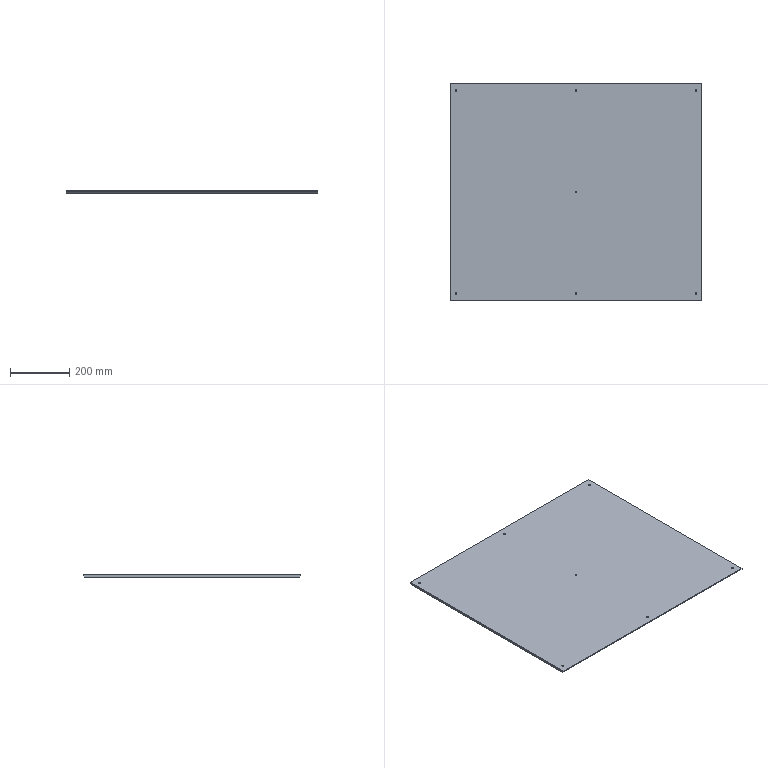Part | SolidWorks | features ICE 4, Chamfer 1, Extrusion 1 | 1 solid | 36 faces | box 850 x 735 x 8 mm | volume 4972189 mm3 | cylinder 14 | cone 14 | plane 8 | commonest cylinder face diameters 6.5 x14
STEP:
#1=CARTESIAN_POINT('',(-3.25,0.,8.));
#2=VERTEX_POINT('',#1);
#3=CARTESIAN_POINT('',(3.25,0.,8.));
#4=VERTEX_POINT('',#3);
#5=CARTESIAN_POINT('',(0.,0.,8.));
#6=DIRECTION('',(0.,0.,1.));
#7=DIRECTION('',(1.,0.,0.));
#8=AXIS2_PLACEMENT_3D('',#5,#6,#7);
#9=CIRCLE('',#8,3.25);
#10=EDGE_CURVE('',#2,#4,#9,.T.);
#11=ORIENTED_EDGE('',*,*,#10,.T.);
#12=CARTESIAN_POINT('',(3.25,0.,5.));
#13=VERTEX_POINT('',#12);
#14=CARTESIAN_POINT('',(3.25,0.,10.));
#15=DIRECTION('',(0.,0.,-1.));
#16=VECTOR('',#15,1000.);
#17=LINE('',#14,#16);
#18=EDGE_CURVE('',#4,#13,#17,.T.);
#19=ORIENTED_EDGE('',*,*,#18,.T.);
#20=CARTESIAN_POINT('',(-3.25,0.,5.));
#21=VERTEX_POINT('',#20);
#22=CARTESIAN_POINT('',(0.,0.,5.));
#23=DIRECTION('',(0.,0.,-1.));
#24=DIRECTION('',(-1.,0.,0.));
#25=AXIS2_PLACEMENT_3D('',#22,#23,#24);
#26=CIRCLE('',#25,3.25);
#27=EDGE_CURVE('',#13,#21,#26,.T.);
#28=ORIENTED_EDGE('',*,*,#27,.T.);
#29=CARTESIAN_POINT('',(-3.25,0.,10.));
#30=DIRECTION('',(0.,0.,-1.));
#31=VECTOR('',#30,1000.);
#32=LINE('',#29,#31);
#33=EDGE_CURVE('',#2,#21,#32,.T.);
#34=ORIENTED_EDGE('',*,*,#33,.F.);
#35=EDGE_LOOP('',(#11,#19,#28,#34));
#36=FACE_OUTER_BOUND('',#35,.T.);
#37=CARTESIAN_POINT('',(0.,0.,10.));
#38=DIRECTION('',(0.,0.,-1.));
#39=DIRECTION('',(-1.,0.,0.));
#40=AXIS2_PLACEMENT_3D('',#37,#38,#39);
#41=CYLINDRICAL_SURFACE('',#40,3.25);
#42=ADVANCED_FACE('',(#36),#41,.F.);
#43=ORIENTED_EDGE('',*,*,#27,.F.);
#44=CARTESIAN_POINT('',(8.25,0.,0.));
#45=VERTEX_POINT('',#44);
#46=CARTESIAN_POINT('',(8.25,0.,0.));
#47=DIRECTION('',(0.7071,0.,-0.7071));
#48=VECTOR('',#47,1000.);
#49=LINE('',#46,#48);
#50=EDGE_CURVE('',#13,#45,#49,.T.);
#51=ORIENTED_EDGE('',*,*,#50,.T.);
#52=CARTESIAN_POINT('',(-8.25,0.,0.));
#53=VERTEX_POINT('',#52);
#54=CARTESIAN_POINT('',(0.,0.,0.));
#55=DIRECTION('',(0.,0.,-1.));
#56=DIRECTION('',(-1.,0.,0.));
#57=AXIS2_PLACEMENT_3D('',#54,#55,#56);
#58=CIRCLE('',#57,8.25);
#59=EDGE_CURVE('',#45,#53,#58,.T.);
#60=ORIENTED_EDGE('',*,*,#59,.T.);
#61=CARTESIAN_POINT('',(-8.25,0.,0.));
#62=DIRECTION('',(-0.7071,0.,-0.7071));
#63=VECTOR('',#62,1000.);
#64=LINE('',#61,#63);
#65=EDGE_CURVE('',#21,#53,#64,.T.);
#66=ORIENTED_EDGE('',*,*,#65,.F.);
#67=EDGE_LOOP('',(#43,#51,#60,#66));
#68=FACE_OUTER_BOUND('',#67,.T.);
#69=CARTESIAN_POINT('',(0.,0.,0.));
#70=DIRECTION('',(0.,0.,-1.));
#71=DIRECTION('',(-1.,0.,0.));
#72=AXIS2_PLACEMENT_3D('',#69,#70,#71);
#73=CONICAL_SURFACE('',#72,8.25,0.7854);
#74=ADVANCED_FACE('',(#68),#73,.F.);
#75=CARTESIAN_POINT('',(-3.25,342.5,5.));
#76=VERTEX_POINT('',#75);
#77=CARTESIAN_POINT('',(3.25,342.5,5.));
#78=VERTEX_POINT('',#77);
#79=CARTESIAN_POINT('',(0.,342.5,5.));
#80=DIRECTION('',(0.,0.,1.));
#81=DIRECTION('',(1.,0.,0.));
#82=AXIS2_PLACEMENT_3D('',#79,#80,#81);
#83=CIRCLE('',#82,3.25);
#84=EDGE_CURVE('',#76,#78,#83,.T.);
#85=ORIENTED_EDGE('',*,*,#84,.F.);
#86=CARTESIAN_POINT('',(-3.25,342.5,8.));
#87=VERTEX_POINT('',#86);
#88=CARTESIAN_POINT('',(-3.25,342.5,5.));
#89=DIRECTION('',(0.,0.,1.));
#90=VECTOR('',#89,1000.);
#91=LINE('',#88,#90);
#92=EDGE_CURVE('',#76,#87,#91,.T.);
#93=ORIENTED_EDGE('',*,*,#92,.T.);
#94=CARTESIAN_POINT('',(3.25,342.5,8.));
#95=VERTEX_POINT('',#94);
#96=CARTESIAN_POINT('',(0.,342.5,8.));
#97=DIRECTION('',(0.,0.,1.));
#98=DIRECTION('',(1.,0.,0.));
#99=AXIS2_PLACEMENT_3D('',#96,#97,#98);
#100=CIRCLE('',#99,3.25);
#101=EDGE_CURVE('',#87,#95,#100,.T.);
#102=ORIENTED_EDGE('',*,*,#101,.T.);
#103=CARTESIAN_POINT('',(3.25,342.5,5.));
#104=DIRECTION('',(0.,0.,1.));
#105=VECTOR('',#104,1000.);
#106=LINE('',#103,#105);
#107=EDGE_CURVE('',#78,#95,#106,.T.);
#108=ORIENTED_EDGE('',*,*,#107,.F.);
#109=EDGE_LOOP('',(#85,#93,#102,#108));
#110=FACE_OUTER_BOUND('',#109,.T.);
#111=CARTESIAN_POINT('',(0.,342.5,5.));
#112=DIRECTION('',(0.,0.,1.));
#113=DIRECTION('',(1.,0.,0.));
#114=AXIS2_PLACEMENT_3D('',#111,#112,#113);
#115=CYLINDRICAL_SURFACE('',#114,3.25);
#116=ADVANCED_FACE('',(#110),#115,.F.);
#117=CARTESIAN_POINT('',(401.75,342.5,5.));
#118=VERTEX_POINT('',#117);
#119=CARTESIAN_POINT('',(408.25,342.5,5.));
#120=VERTEX_POINT('',#119);
#121=CARTESIAN_POINT('',(405.,342.5,5.));
#122=DIRECTION('',(0.,0.,1.));
#123=DIRECTION('',(1.,0.,0.));
#124=AXIS2_PLACEMENT_3D('',#121,#122,#123);
#125=CIRCLE('',#124,3.25);
#126=EDGE_CURVE('',#118,#120,#125,.T.);
#127=ORIENTED_EDGE('',*,*,#126,.F.);
#128=CARTESIAN_POINT('',(401.75,342.5,8.));
#129=VERTEX_POINT('',#128);
#130=CARTESIAN_POINT('',(401.75,342.5,5.));
#131=DIRECTION('',(0.,0.,1.));
#132=VECTOR('',#131,1000.);
#133=LINE('',#130,#132);
#134=EDGE_CURVE('',#118,#129,#133,.T.);
#135=ORIENTED_EDGE('',*,*,#134,.T.);
#136=CARTESIAN_POINT('',(408.25,342.5,8.));
#137=VERTEX_POINT('',#136);
#138=CARTESIAN_POINT('',(405.,342.5,8.));
#139=DIRECTION('',(0.,0.,1.));
#140=DIRECTION('',(1.,0.,0.));
#141=AXIS2_PLACEMENT_3D('',#138,#139,#140);
#142=CIRCLE('',#141,3.25);
#143=EDGE_CURVE('',#129,#137,#142,.T.);
#144=ORIENTED_EDGE('',*,*,#143,.T.);
#145=CARTESIAN_POINT('',(408.25,342.5,5.));
#146=DIRECTION('',(0.,0.,1.));
#147=VECTOR('',#146,1000.);
#148=LINE('',#145,#147);
#149=EDGE_CURVE('',#120,#137,#148,.T.);
#150=ORIENTED_EDGE('',*,*,#149,.F.);
#151=EDGE_LOOP('',(#127,#135,#144,#150));
#152=FACE_OUTER_BOUND('',#151,.T.);
#153=CARTESIAN_POINT('',(405.,342.5,5.));
#154=DIRECTION('',(0.,0.,1.));
#155=DIRECTION('',(1.,0.,0.));
#156=AXIS2_PLACEMENT_3D('',#153,#154,#155);
#157=CYLINDRICAL_SURFACE('',#156,3.25);
#158=ADVANCED_FACE('',(#152),#157,.F.);
#159=CARTESIAN_POINT('',(-408.25,-342.5,5.));
#160=VERTEX_POINT('',#159);
#161=CARTESIAN_POINT('',(-401.75,-342.5,5.));
#162=VERTEX_POINT('',#161);
#163=CARTESIAN_POINT('',(-405.,-342.5,5.));
#164=DIRECTION('',(0.,0.,1.));
#165=DIRECTION('',(1.,0.,0.));
#166=AXIS2_PLACEMENT_3D('',#163,#164,#165);
#167=CIRCLE('',#166,3.25);
#168=EDGE_CURVE('',#160,#162,#167,.T.);
#169=ORIENTED_EDGE('',*,*,#168,.F.);
#170=CARTESIAN_POINT('',(-408.25,-342.5,8.));
#171=VERTEX_POINT('',#170);
#172=CARTESIAN_POINT('',(-408.25,-342.5,5.));
#173=DIRECTION('',(0.,0.,1.));
#174=VECTOR('',#173,1000.);
#175=LINE('',#172,#174);
#176=EDGE_CURVE('',#160,#171,#175,.T.);
#177=ORIENTED_EDGE('',*,*,#176,.T.);
#178=CARTESIAN_POINT('',(-401.75,-342.5,8.));
#179=VERTEX_POINT('',#178);
#180=CARTESIAN_POINT('',(-405.,-342.5,8.));
#181=DIRECTION('',(0.,0.,1.));
#182=DIRECTION('',(1.,0.,0.));
#183=AXIS2_PLACEMENT_3D('',#180,#181,#182);
#184=CIRCLE('',#183,3.25);
#185=EDGE_CURVE('',#171,#179,#184,.T.);
#186=ORIENTED_EDGE('',*,*,#185,.T.);
#187=CARTESIAN_POINT('',(-401.75,-342.5,5.));
#188=DIRECTION('',(0.,0.,1.));
#189=VECTOR('',#188,1000.);
#190=LINE('',#187,#189);
#191=EDGE_CURVE('',#162,#179,#190,.T.);
#192=ORIENTED_EDGE('',*,*,#191,.F.);
#193=EDGE_LOOP('',(#169,#177,#186,#192));
#194=FACE_OUTER_BOUND('',#193,.T.);
#195=CARTESIAN_POINT('',(-405.,-342.5,5.));
#196=DIRECTION('',(0.,0.,1.));
#197=DIRECTION('',(1.,0.,0.));
#198=AXIS2_PLACEMENT_3D('',#195,#196,#197);
#199=CYLINDRICAL_SURFACE('',#198,3.25);
#200=ADVANCED_FACE('',(#194),#199,.F.);
#201=CARTESIAN_POINT('',(-3.25,-342.5,5.));
#202=VERTEX_POINT('',#201);
#203=CARTESIAN_POINT('',(3.25,-342.5,5.));
#204=VERTEX_POINT('',#203);
#205=CARTESIAN_POINT('',(0.,-342.5,5.));
#206=DIRECTION('',(0.,0.,1.));
#207=DIRECTION('',(1.,0.,0.));
#208=AXIS2_PLACEMENT_3D('',#205,#206,#207);
#209=CIRCLE('',#208,3.25);
#210=EDGE_CURVE('',#202,#204,#209,.T.);
#211=ORIENTED_EDGE('',*,*,#210,.F.);
#212=CARTESIAN_POINT('',(-3.25,-342.5,8.));
#213=VERTEX_POINT('',#212);
#214=CARTESIAN_POINT('',(-3.25,-342.5,5.));
#215=DIRECTION('',(0.,0.,1.));
#216=VECTOR('',#215,1000.);
#217=LINE('',#214,#216);
#218=EDGE_CURVE('',#202,#213,#217,.T.);
#219=ORIENTED_EDGE('',*,*,#218,.T.);
#220=CARTESIAN_POINT('',(3.25,-342.5,8.));
#221=VERTEX_POINT('',#220);
#222=CARTESIAN_POINT('',(0.,-342.5,8.));
#223=DIRECTION('',(0.,0.,1.));
#224=DIRECTION('',(1.,0.,0.));
#225=AXIS2_PLACEMENT_3D('',#222,#223,#224);
#226=CIRCLE('',#225,3.25);
#227=EDGE_CURVE('',#213,#221,#226,.T.);
#228=ORIENTED_EDGE('',*,*,#227,.T.);
#229=CARTESIAN_POINT('',(3.25,-342.5,5.));
#230=DIRECTION('',(0.,0.,1.));
#231=VECTOR('',#230,1000.);
#232=LINE('',#229,#231);
#233=EDGE_CURVE('',#204,#221,#232,.T.);
#234=ORIENTED_EDGE('',*,*,#233,.F.);
#235=EDGE_LOOP('',(#211,#219,#228,#234));
#236=FACE_OUTER_BOUND('',#235,.T.);
#237=CARTESIAN_POINT('',(0.,-342.5,5.));
#238=DIRECTION('',(0.,0.,1.));
#239=DIRECTION('',(1.,0.,0.));
#240=AXIS2_PLACEMENT_3D('',#237,#238,#239);
#241=CYLINDRICAL_SURFACE('',#240,3.25);
#242=ADVANCED_FACE('',(#236),#241,.F.);
#243=CARTESIAN_POINT('',(401.75,-342.5,5.));
#244=VERTEX_POINT('',#243);
#245=CARTESIAN_POINT('',(408.25,-342.5,5.));
#246=VERTEX_POINT('',#245);
#247=CARTESIAN_POINT('',(405.,-342.5,5.));
#248=DIRECTION('',(0.,0.,1.));
#249=DIRECTION('',(1.,0.,0.));
#250=AXIS2_PLACEMENT_3D('',#247,#248,#249);
#251=CIRCLE('',#250,3.25);
#252=EDGE_CURVE('',#244,#246,#251,.T.);
#253=ORIENTED_EDGE('',*,*,#252,.F.);
#254=CARTESIAN_POINT('',(401.75,-342.5,8.));
#255=VERTEX_POINT('',#254);
#256=CARTESIAN_POINT('',(401.75,-342.5,5.));
#257=DIRECTION('',(0.,0.,1.));
#258=VECTOR('',#257,1000.);
#259=LINE('',#256,#258);
#260=EDGE_CURVE('',#244,#255,#259,.T.);
#261=ORIENTED_EDGE('',*,*,#260,.T.);
#262=CARTESIAN_POINT('',(408.25,-342.5,8.));
#263=VERTEX_POINT('',#262);
#264=CARTESIAN_POINT('',(405.,-342.5,8.));
#265=DIRECTION('',(0.,0.,1.));
#266=DIRECTION('',(1.,0.,0.));
#267=AXIS2_PLACEMENT_3D('',#264,#265,#266);
#268=CIRCLE('',#267,3.25);
#269=EDGE_CURVE('',#255,#263,#268,.T.);
#270=ORIENTED_EDGE('',*,*,#269,.T.);
#271=CARTESIAN_POINT('',(408.25,-342.5,5.));
#272=DIRECTION('',(0.,0.,1.));
#273=VECTOR('',#272,1000.);
#274=LINE('',#271,#273);
#275=EDGE_CURVE('',#246,#263,#274,.T.);
#276=ORIENTED_EDGE('',*,*,#275,.F.);
#277=EDGE_LOOP('',(#253,#261,#270,#276));
#278=FACE_OUTER_BOUND('',#277,.T.);
#279=CARTESIAN_POINT('',(405.,-342.5,5.));
#280=DIRECTION('',(0.,0.,1.));
#281=DIRECTION('',(1.,0.,0.));
#282=AXIS2_PLACEMENT_3D('',#279,#280,#281);
#283=CYLINDRICAL_SURFACE('',#282,3.25);
#284=ADVANCED_FACE('',(#278),#283,.F.);
#285=CARTESIAN_POINT('',(-408.25,342.5,5.));
#286=VERTEX_POINT('',#285);
#287=CARTESIAN_POINT('',(-401.75,342.5,5.));
#288=VERTEX_POINT('',#287);
#289=CARTESIAN_POINT('',(-405.,342.5,5.));
#290=DIRECTION('',(0.,0.,1.));
#291=DIRECTION('',(1.,0.,0.));
#292=AXIS2_PLACEMENT_3D('',#289,#290,#291);
#293=CIRCLE('',#292,3.25);
#294=EDGE_CURVE('',#286,#288,#293,.T.);
#295=ORIENTED_EDGE('',*,*,#294,.F.);
#296=CARTESIAN_POINT('',(-408.25,342.5,8.));
#297=VERTEX_POINT('',#296);
#298=CARTESIAN_POINT('',(-408.25,342.5,5.));
#299=DIRECTION('',(0.,0.,1.));
#300=VECTOR('',#299,1000.);
#301=LINE('',#298,#300);
#302=EDGE_CURVE('',#286,#297,#301,.T.);
#303=ORIENTED_EDGE('',*,*,#302,.T.);
#304=CARTESIAN_POINT('',(-401.75,342.5,8.));
#305=VERTEX_POINT('',#304);
#306=CARTESIAN_POINT('',(-405.,342.5,8.));
#307=DIRECTION('',(0.,0.,1.));
#308=DIRECTION('',(1.,0.,0.));
#309=AXIS2_PLACEMENT_3D('',#306,#307,#308);
#310=CIRCLE('',#309,3.25);
#311=EDGE_CURVE('',#297,#305,#310,.T.);
#312=ORIENTED_EDGE('',*,*,#311,.T.);
#313=CARTESIAN_POINT('',(-401.75,342.5,5.));
#314=DIRECTION('',(0.,0.,1.));
#315=VECTOR('',#314,1000.);
#316=LINE('',#313,#315);
#317=EDGE_CURVE('',#288,#305,#316,.T.);
#318=ORIENTED_EDGE('',*,*,#317,.F.);
#319=EDGE_LOOP('',(#295,#303,#312,#318));
#320=FACE_OUTER_BOUND('',#319,.T.);
#321=CARTESIAN_POINT('',(-405.,342.5,5.));
#322=DIRECTION('',(0.,0.,1.));
#323=DIRECTION('',(1.,0.,0.));
#324=AXIS2_PLACEMENT_3D('',#321,#322,#323);
#325=CYLINDRICAL_SURFACE('',#324,3.25);
#326=ADVANCED_FACE('',(#320),#325,.F.);
#327=ORIENTED_EDGE('',*,*,#84,.T.);
#328=CARTESIAN_POINT('',(8.25,342.5,0.));
#329=VERTEX_POINT('',#328);
#330=CARTESIAN_POINT('',(8.25,342.5,0.));
#331=DIRECTION('',(0.7071,0.,-0.7071));
#332=VECTOR('',#331,1000.);
#333=LINE('',#330,#332);
#334=EDGE_CURVE('',#78,#329,#333,.T.);
#335=ORIENTED_EDGE('',*,*,#334,.T.);
#336=CARTESIAN_POINT('',(-8.25,342.5,0.));
#337=VERTEX_POINT('',#336);
#338=CARTESIAN_POINT('',(0.,342.5,0.));
#339=DIRECTION('',(0.,0.,-1.));
#340=DIRECTION('',(-1.,0.,0.));
#341=AXIS2_PLACEMENT_3D('',#338,#339,#340);
#342=CIRCLE('',#341,8.25);
#343=EDGE_CURVE('',#329,#337,#342,.T.);
#344=ORIENTED_EDGE('',*,*,#343,.T.);
#345=CARTESIAN_POINT('',(-8.25,342.5,0.));
#346=DIRECTION('',(-0.7071,0.,-0.7071));
#347=VECTOR('',#346,1000.);
#348=LINE('',#345,#347);
#349=EDGE_CURVE('',#76,#337,#348,.T.);
#350=ORIENTED_EDGE('',*,*,#349,.F.);
#351=EDGE_LOOP('',(#327,#335,#344,#350));
#352=FACE_OUTER_BOUND('',#351,.T.);
#353=CARTESIAN_POINT('',(0.,342.5,0.));
#354=DIRECTION('',(0.,0.,-1.));
#355=DIRECTION('',(-1.,0.,0.));
#356=AXIS2_PLACEMENT_3D('',#353,#354,#355);
#357=CONICAL_SURFACE('',#356,8.25,0.7854);
#358=ADVANCED_FACE('',(#352),#357,.F.);
#359=ORIENTED_EDGE('',*,*,#294,.T.);
#360=CARTESIAN_POINT('',(-396.75,342.5,0.));
#361=VERTEX_POINT('',#360);
#362=CARTESIAN_POINT('',(-396.75,342.5,0.));
#363=DIRECTION('',(0.7071,0.,-0.7071));
#364=VECTOR('',#363,1000.);
#365=LINE('',#362,#364);
#366=EDGE_CURVE('',#288,#361,#365,.T.);
#367=ORIENTED_EDGE('',*,*,#366,.T.);
#368=CARTESIAN_POINT('',(-413.25,342.5,0.));
#369=VERTEX_POINT('',#368);
#370=CARTESIAN_POINT('',(-405.,342.5,0.));
#371=DIRECTION('',(0.,0.,-1.));
#372=DIRECTION('',(-1.,0.,0.));
#373=AXIS2_PLACEMENT_3D('',#370,#371,#372);
#374=CIRCLE('',#373,8.25);
#375=EDGE_CURVE('',#361,#369,#374,.T.);
#376=ORIENTED_EDGE('',*,*,#375,.T.);
#377=CARTESIAN_POINT('',(-413.25,342.5,0.));
#378=DIRECTION('',(-0.7071,0.,-0.7071));
#379=VECTOR('',#378,1000.);
#380=LINE('',#377,#379);
#381=EDGE_CURVE('',#286,#369,#380,.T.);
#382=ORIENTED_EDGE('',*,*,#381,.F.);
#383=EDGE_LOOP('',(#359,#367,#376,#382));
#384=FACE_OUTER_BOUND('',#383,.T.);
#385=CARTESIAN_POINT('',(-405.,342.5,0.));
#386=DIRECTION('',(0.,0.,-1.));
#387=DIRECTION('',(-1.,0.,0.));
#388=AXIS2_PLACEMENT_3D('',#385,#386,#387);
#389=CONICAL_SURFACE('',#388,8.25,0.7854);
#390=ADVANCED_FACE('',(#384),#389,.F.);
#391=ORIENTED_EDGE('',*,*,#252,.T.);
#392=CARTESIAN_POINT('',(413.25,-342.5,0.));
#393=VERTEX_POINT('',#392);
#394=CARTESIAN_POINT('',(413.25,-342.5,0.));
#395=DIRECTION('',(0.7071,0.,-0.7071));
#396=VECTOR('',#395,1000.);
#397=LINE('',#394,#396);
#398=EDGE_CURVE('',#246,#393,#397,.T.);
#399=ORIENTED_EDGE('',*,*,#398,.T.);
#400=CARTESIAN_POINT('',(396.75,-342.5,0.));
#401=VERTEX_POINT('',#400);
#402=CARTESIAN_POINT('',(405.,-342.5,0.));
#403=DIRECTION('',(0.,0.,-1.));
#404=DIRECTION('',(-1.,0.,0.));
#405=AXIS2_PLACEMENT_3D('',#402,#403,#404);
#406=CIRCLE('',#405,8.25);
#407=EDGE_CURVE('',#393,#401,#406,.T.);
#408=ORIENTED_EDGE('',*,*,#407,.T.);
#409=CARTESIAN_POINT('',(396.75,-342.5,0.));
#410=DIRECTION('',(-0.7071,0.,-0.7071));
#411=VECTOR('',#410,1000.);
#412=LINE('',#409,#411);
#413=EDGE_CURVE('',#244,#401,#412,.T.);
#414=ORIENTED_EDGE('',*,*,#413,.F.);
#415=EDGE_LOOP('',(#391,#399,#408,#414));
#416=FACE_OUTER_BOUND('',#415,.T.);
#417=CARTESIAN_POINT('',(405.,-342.5,0.));
#418=DIRECTION('',(0.,0.,-1.));
#419=DIRECTION('',(-1.,0.,0.));
#420=AXIS2_PLACEMENT_3D('',#417,#418,#419);
#421=CONICAL_SURFACE('',#420,8.25,0.7854);
#422=ADVANCED_FACE('',(#416),#421,.F.);
#423=ORIENTED_EDGE('',*,*,#210,.T.);
#424=CARTESIAN_POINT('',(8.25,-342.5,0.));
#425=VERTEX_POINT('',#424);
#426=CARTESIAN_POINT('',(8.25,-342.5,0.));
#427=DIRECTION('',(0.7071,0.,-0.7071));
#428=VECTOR('',#427,1000.);
#429=LINE('',#426,#428);
#430=EDGE_CURVE('',#204,#425,#429,.T.);
#431=ORIENTED_EDGE('',*,*,#430,.T.);
#432=CARTESIAN_POINT('',(-8.25,-342.5,0.));
#433=VERTEX_POINT('',#432);
#434=CARTESIAN_POINT('',(0.,-342.5,0.));
#435=DIRECTION('',(0.,0.,-1.));
#436=DIRECTION('',(-1.,0.,0.));
#437=AXIS2_PLACEMENT_3D('',#434,#435,#436);
#438=CIRCLE('',#437,8.25);
#439=EDGE_CURVE('',#425,#433,#438,.T.);
#440=ORIENTED_EDGE('',*,*,#439,.T.);
#441=CARTESIAN_POINT('',(-8.25,-342.5,0.));
#442=DIRECTION('',(-0.7071,0.,-0.7071));
#443=VECTOR('',#442,1000.);
#444=LINE('',#441,#443);
#445=EDGE_CURVE('',#202,#433,#444,.T.);
#446=ORIENTED_EDGE('',*,*,#445,.F.);
#447=EDGE_LOOP('',(#423,#431,#440,#446));
#448=FACE_OUTER_BOUND('',#447,.T.);
#449=CARTESIAN_POINT('',(0.,-342.5,0.));
#450=DIRECTION('',(0.,0.,-1.));
#451=DIRECTION('',(-1.,0.,0.));
#452=AXIS2_PLACEMENT_3D('',#449,#450,#451);
#453=CONICAL_SURFACE('',#452,8.25,0.7854);
#454=ADVANCED_FACE('',(#448),#453,.F.);
#455=ORIENTED_EDGE('',*,*,#168,.T.);
#456=CARTESIAN_POINT('',(-396.75,-342.5,0.));
#457=VERTEX_POINT('',#456);
#458=CARTESIAN_POINT('',(-396.75,-342.5,0.));
#459=DIRECTION('',(0.7071,0.,-0.7071));
#460=VECTOR('',#459,1000.);
#461=LINE('',#458,#460);
#462=EDGE_CURVE('',#162,#457,#461,.T.);
#463=ORIENTED_EDGE('',*,*,#462,.T.);
#464=CARTESIAN_POINT('',(-413.25,-342.5,0.));
#465=VERTEX_POINT('',#464);
#466=CARTESIAN_POINT('',(-405.,-342.5,0.));
#467=DIRECTION('',(0.,0.,-1.));
#468=DIRECTION('',(-1.,0.,0.));
#469=AXIS2_PLACEMENT_3D('',#466,#467,#468);
#470=CIRCLE('',#469,8.25);
#471=EDGE_CURVE('',#457,#465,#470,.T.);
#472=ORIENTED_EDGE('',*,*,#471,.T.);
#473=CARTESIAN_POINT('',(-413.25,-342.5,0.));
#474=DIRECTION('',(-0.7071,0.,-0.7071));
#475=VECTOR('',#474,1000.);
#476=LINE('',#473,#475);
#477=EDGE_CURVE('',#160,#465,#476,.T.);
#478=ORIENTED_EDGE('',*,*,#477,.F.);
#479=EDGE_LOOP('',(#455,#463,#472,#478));
#480=FACE_OUTER_BOUND('',#479,.T.);
#481=CARTESIAN_POINT('',(-405.,-342.5,0.));
#482=DIRECTION('',(0.,0.,-1.));
#483=DIRECTION('',(-1.,0.,0.));
#484=AXIS2_PLACEMENT_3D('',#481,#482,#483);
#485=CONICAL_SURFACE('',#484,8.25,0.7854);
#486=ADVANCED_FACE('',(#480),#485,.F.);
#487=ORIENTED_EDGE('',*,*,#126,.T.);
#488=CARTESIAN_POINT('',(413.25,342.5,0.));
#489=VERTEX_POINT('',#488);
#490=CARTESIAN_POINT('',(413.25,342.5,0.));
#491=DIRECTION('',(0.7071,0.,-0.7071));
#492=VECTOR('',#491,1000.);
#493=LINE('',#490,#492);
#494=EDGE_CURVE('',#120,#489,#493,.T.);
#495=ORIENTED_EDGE('',*,*,#494,.T.);
#496=CARTESIAN_POINT('',(396.75,342.5,0.));
#497=VERTEX_POINT('',#496);
#498=CARTESIAN_POINT('',(405.,342.5,0.));
#499=DIRECTION('',(0.,0.,-1.));
#500=DIRECTION('',(-1.,0.,0.));
#501=AXIS2_PLACEMENT_3D('',#498,#499,#500);
#502=CIRCLE('',#501,8.25);
#503=EDGE_CURVE('',#489,#497,#502,.T.);
#504=ORIENTED_EDGE('',*,*,#503,.T.);
#505=CARTESIAN_POINT('',(396.75,342.5,0.));
#506=DIRECTION('',(-0.7071,0.,-0.7071));
#507=VECTOR('',#506,1000.);
#508=LINE('',#505,#507);
#509=EDGE_CURVE('',#118,#497,#508,.T.);
#510=ORIENTED_EDGE('',*,*,#509,.F.);
#511=EDGE_LOOP('',(#487,#495,#504,#510));
#512=FACE_OUTER_BOUND('',#511,.T.);
#513=CARTESIAN_POINT('',(405.,342.5,0.));
#514=DIRECTION('',(0.,0.,-1.));
#515=DIRECTION('',(-1.,0.,0.));
#516=AXIS2_PLACEMENT_3D('',#513,#514,#515);
#517=CONICAL_SURFACE('',#516,8.25,0.7854);
#518=ADVANCED_FACE('',(#512),#517,.F.);
#519=CARTESIAN_POINT('',(425.,-367.5,8.));
#520=VERTEX_POINT('',#519);
#521=CARTESIAN_POINT('',(425.,-367.5,5.));
#522=VERTEX_POINT('',#521);
#523=CARTESIAN_POINT('',(425.,-367.5,8.));
#524=DIRECTION('',(0.,0.,-1.));
#525=VECTOR('',#524,1000.);
#526=LINE('',#523,#525);
#527=EDGE_CURVE('',#520,#522,#526,.T.);
#528=ORIENTED_EDGE('',*,*,#527,.T.);
#529=CARTESIAN_POINT('',(425.,-362.5,0.));
#530=VERTEX_POINT('',#529);
#531=CARTESIAN_POINT('',(425.,-367.5,5.));
#532=DIRECTION('',(0.,0.7071,-0.7071));
#533=VECTOR('',#532,1000.);
#534=LINE('',#531,#533);
#535=EDGE_CURVE('',#522,#530,#534,.T.);
#536=ORIENTED_EDGE('',*,*,#535,.T.);
#537=CARTESIAN_POINT('',(425.,362.5,0.));
#538=VERTEX_POINT('',#537);
#539=CARTESIAN_POINT('',(425.,367.5,0.));
#540=DIRECTION('',(0.,1.,0.));
#541=VECTOR('',#540,1000.);
#542=LINE('',#539,#541);
#543=EDGE_CURVE('',#530,#538,#542,.T.);
#544=ORIENTED_EDGE('',*,*,#543,.T.);
#545=CARTESIAN_POINT('',(425.,367.5,5.));
#546=VERTEX_POINT('',#545);
#547=CARTESIAN_POINT('',(425.,367.5,5.));
#548=DIRECTION('',(0.,0.7071,0.7071));
#549=VECTOR('',#548,1000.);
#550=LINE('',#547,#549);
#551=EDGE_CURVE('',#538,#546,#550,.T.);
#552=ORIENTED_EDGE('',*,*,#551,.T.);
#553=CARTESIAN_POINT('',(425.,367.5,8.));
#554=VERTEX_POINT('',#553);
#555=CARTESIAN_POINT('',(425.,367.5,8.));
#556=DIRECTION('',(0.,0.,-1.));
#557=VECTOR('',#556,1000.);
#558=LINE('',#555,#557);
#559=EDGE_CURVE('',#554,#546,#558,.T.);
#560=ORIENTED_EDGE('',*,*,#559,.F.);
#561=CARTESIAN_POINT('',(425.,367.5,8.));
#562=DIRECTION('',(0.,1.,0.));
#563=VECTOR('',#562,1000.);
#564=LINE('',#561,#563);
#565=EDGE_CURVE('',#520,#554,#564,.T.);
#566=ORIENTED_EDGE('',*,*,#565,.F.);
#567=EDGE_LOOP('',(#528,#536,#544,#552,#560,#566));
#568=FACE_OUTER_BOUND('',#567,.T.);
#569=CARTESIAN_POINT('',(425.,367.5,8.));
#570=DIRECTION('',(-1.,0.,0.));
#571=DIRECTION('',(0.,-1.,0.));
#572=AXIS2_PLACEMENT_3D('',#569,#570,#571);
#573=PLANE('',#572);
#574=ADVANCED_FACE('',(#568),#573,.F.);
#575=ORIENTED_EDGE('',*,*,#559,.T.);
#576=CARTESIAN_POINT('',(-425.,367.5,5.));
#577=VERTEX_POINT('',#576);
#578=CARTESIAN_POINT('',(-425.,367.5,5.));
#579=DIRECTION('',(-1.,0.,0.));
#580=VECTOR('',#579,1000.);
#581=LINE('',#578,#580);
#582=EDGE_CURVE('',#546,#577,#581,.T.);
#583=ORIENTED_EDGE('',*,*,#582,.T.);
#584=CARTESIAN_POINT('',(-425.,367.5,8.));
#585=VERTEX_POINT('',#584);
#586=CARTESIAN_POINT('',(-425.,367.5,8.));
#587=DIRECTION('',(0.,0.,-1.));
#588=VECTOR('',#587,1000.);
#589=LINE('',#586,#588);
#590=EDGE_CURVE('',#585,#577,#589,.T.);
#591=ORIENTED_EDGE('',*,*,#590,.F.);
#592=CARTESIAN_POINT('',(-425.,367.5,8.));
#593=DIRECTION('',(-1.,0.,0.));
#594=VECTOR('',#593,1000.);
#595=LINE('',#592,#594);
#596=EDGE_CURVE('',#554,#585,#595,.T.);
#597=ORIENTED_EDGE('',*,*,#596,.F.);
#598=EDGE_LOOP('',(#575,#583,#591,#597));
#599=FACE_OUTER_BOUND('',#598,.T.);
#600=CARTESIAN_POINT('',(-425.,367.5,8.));
#601=DIRECTION('',(0.,-1.,0.));
#602=DIRECTION('',(0.,0.,-1.));
#603=AXIS2_PLACEMENT_3D('',#600,#601,#602);
#604=PLANE('',#603);
#605=ADVANCED_FACE('',(#599),#604,.F.);
#606=CARTESIAN_POINT('',(-425.,362.5,0.));
#607=VERTEX_POINT('',#606);
#608=CARTESIAN_POINT('',(-425.,-362.5,0.));
#609=VERTEX_POINT('',#608);
#610=CARTESIAN_POINT('',(-425.,367.5,0.));
#611=DIRECTION('',(0.,-1.,0.));
#612=VECTOR('',#611,1000.);
#613=LINE('',#610,#612);
#614=EDGE_CURVE('',#607,#609,#613,.T.);
#615=ORIENTED_EDGE('',*,*,#614,.T.);
#616=CARTESIAN_POINT('',(-425.,-367.5,5.));
#617=VERTEX_POINT('',#616);
#618=CARTESIAN_POINT('',(-425.,-367.5,5.));
#619=DIRECTION('',(0.,-0.7071,0.7071));
#620=VECTOR('',#619,1000.);
#621=LINE('',#618,#620);
#622=EDGE_CURVE('',#609,#617,#621,.T.);
#623=ORIENTED_EDGE('',*,*,#622,.T.);
#624=CARTESIAN_POINT('',(-425.,-367.5,8.));
#625=VERTEX_POINT('',#624);
#626=CARTESIAN_POINT('',(-425.,-367.5,8.));
#627=DIRECTION('',(0.,0.,-1.));
#628=VECTOR('',#627,1000.);
#629=LINE('',#626,#628);
#630=EDGE_CURVE('',#625,#617,#629,.T.);
#631=ORIENTED_EDGE('',*,*,#630,.F.);
#632=CARTESIAN_POINT('',(-425.,367.5,8.));
#633=DIRECTION('',(0.,-1.,0.));
#634=VECTOR('',#633,1000.);
#635=LINE('',#632,#634);
#636=EDGE_CURVE('',#585,#625,#635,.T.);
#637=ORIENTED_EDGE('',*,*,#636,.F.);
#638=ORIENTED_EDGE('',*,*,#590,.T.);
#639=CARTESIAN_POINT('',(-425.,367.5,5.));
#640=DIRECTION('',(0.,-0.7071,-0.7071));
#641=VECTOR('',#640,1000.);
#642=LINE('',#639,#641);
#643=EDGE_CURVE('',#577,#607,#642,.T.);
#644=ORIENTED_EDGE('',*,*,#643,.T.);
#645=EDGE_LOOP('',(#615,#623,#631,#637,#638,#644));
#646=FACE_OUTER_BOUND('',#645,.T.);
#647=CARTESIAN_POINT('',(-425.,367.5,8.));
#648=DIRECTION('',(1.,0.,0.));
#649=DIRECTION('',(0.,1.,0.));
#650=AXIS2_PLACEMENT_3D('',#647,#648,#649);
#651=PLANE('',#650);
#652=ADVANCED_FACE('',(#646),#651,.F.);
#653=ORIENTED_EDGE('',*,*,#630,.T.);
#654=CARTESIAN_POINT('',(-425.,-367.5,5.));
#655=DIRECTION('',(1.,0.,0.));
#656=VECTOR('',#655,1000.);
#657=LINE('',#654,#656);
#658=EDGE_CURVE('',#617,#522,#657,.T.);
#659=ORIENTED_EDGE('',*,*,#658,.T.);
#660=ORIENTED_EDGE('',*,*,#527,.F.);
#661=CARTESIAN_POINT('',(-425.,-367.5,8.));
#662=DIRECTION('',(1.,0.,0.));
#663=VECTOR('',#662,1000.);
#664=LINE('',#661,#663);
#665=EDGE_CURVE('',#625,#520,#664,.T.);
#666=ORIENTED_EDGE('',*,*,#665,.F.);
#667=EDGE_LOOP('',(#653,#659,#660,#666));
#668=FACE_OUTER_BOUND('',#667,.T.);
#669=CARTESIAN_POINT('',(-425.,-367.5,8.));
#670=DIRECTION('',(0.,1.,0.));
#671=DIRECTION('',(0.,0.,1.));
#672=AXIS2_PLACEMENT_3D('',#669,#670,#671);
#673=PLANE('',#672);
#674=ADVANCED_FACE('',(#668),#673,.F.);
#675=ORIENTED_EDGE('',*,*,#10,.F.);
#676=CARTESIAN_POINT('',(0.,0.,8.));
#677=DIRECTION('',(0.,0.,1.));
#678=DIRECTION('',(1.,0.,0.));
#679=AXIS2_PLACEMENT_3D('',#676,#677,#678);
#680=CIRCLE('',#679,3.25);
#681=EDGE_CURVE('',#4,#2,#680,.T.);
#682=ORIENTED_EDGE('',*,*,#681,.F.);
#683=EDGE_LOOP('',(#675,#682));
#684=FACE_BOUND('',#683,.T.);
#685=CARTESIAN_POINT('',(0.,342.5,8.));
#686=DIRECTION('',(0.,0.,1.));
#687=DIRECTION('',(1.,0.,0.));
#688=AXIS2_PLACEMENT_3D('',#685,#686,#687);
#689=CIRCLE('',#688,3.25);
#690=EDGE_CURVE('',#95,#87,#689,.T.);
#691=ORIENTED_EDGE('',*,*,#690,.F.);
#692=ORIENTED_EDGE('',*,*,#101,.F.);
#693=EDGE_LOOP('',(#691,#692));
#694=FACE_BOUND('',#693,.T.);
#695=CARTESIAN_POINT('',(405.,342.5,8.));
#696=DIRECTION('',(0.,0.,1.));
#697=DIRECTION('',(1.,0.,0.));
#698=AXIS2_PLACEMENT_3D('',#695,#696,#697);
#699=CIRCLE('',#698,3.25);
#700=EDGE_CURVE('',#137,#129,#699,.T.);
#701=ORIENTED_EDGE('',*,*,#700,.F.);
#702=ORIENTED_EDGE('',*,*,#143,.F.);
#703=EDGE_LOOP('',(#701,#702));
#704=FACE_BOUND('',#703,.T.);
#705=CARTESIAN_POINT('',(-405.,-342.5,8.));
#706=DIRECTION('',(0.,0.,1.));
#707=DIRECTION('',(1.,0.,0.));
#708=AXIS2_PLACEMENT_3D('',#705,#706,#707);
#709=CIRCLE('',#708,3.25);
#710=EDGE_CURVE('',#179,#171,#709,.T.);
#711=ORIENTED_EDGE('',*,*,#710,.F.);
#712=ORIENTED_EDGE('',*,*,#185,.F.);
#713=EDGE_LOOP('',(#711,#712));
#714=FACE_BOUND('',#713,.T.);
#715=CARTESIAN_POINT('',(0.,-342.5,8.));
#716=DIRECTION('',(0.,0.,1.));
#717=DIRECTION('',(1.,0.,0.));
#718=AXIS2_PLACEMENT_3D('',#715,#716,#717);
#719=CIRCLE('',#718,3.25);
#720=EDGE_CURVE('',#221,#213,#719,.T.);
#721=ORIENTED_EDGE('',*,*,#720,.F.);
#722=ORIENTED_EDGE('',*,*,#227,.F.);
#723=EDGE_LOOP('',(#721,#722));
#724=FACE_BOUND('',#723,.T.);
#725=CARTESIAN_POINT('',(405.,-342.5,8.));
#726=DIRECTION('',(0.,0.,1.));
#727=DIRECTION('',(1.,0.,0.));
#728=AXIS2_PLACEMENT_3D('',#725,#726,#727);
#729=CIRCLE('',#728,3.25);
#730=EDGE_CURVE('',#263,#255,#729,.T.);
#731=ORIENTED_EDGE('',*,*,#730,.F.);
#732=ORIENTED_EDGE('',*,*,#269,.F.);
#733=EDGE_LOOP('',(#731,#732));
#734=FACE_BOUND('',#733,.T.);
#735=CARTESIAN_POINT('',(-405.,342.5,8.));
#736=DIRECTION('',(0.,0.,1.));
#737=DIRECTION('',(1.,0.,0.));
#738=AXIS2_PLACEMENT_3D('',#735,#736,#737);
#739=CIRCLE('',#738,3.25);
#740=EDGE_CURVE('',#305,#297,#739,.T.);
#741=ORIENTED_EDGE('',*,*,#740,.F.);
#742=ORIENTED_EDGE('',*,*,#311,.F.);
#743=EDGE_LOOP('',(#741,#742));
#744=FACE_BOUND('',#743,.T.);
#745=ORIENTED_EDGE('',*,*,#565,.T.);
#746=ORIENTED_EDGE('',*,*,#596,.T.);
#747=ORIENTED_EDGE('',*,*,#636,.T.);
#748=ORIENTED_EDGE('',*,*,#665,.T.);
#749=EDGE_LOOP('',(#745,#746,#747,#748));
#750=FACE_OUTER_BOUND('',#749,.T.);
#751=CARTESIAN_POINT('',(0.,0.,8.));
#752=DIRECTION('',(0.,0.,1.));
#753=DIRECTION('',(1.,0.,0.));
#754=AXIS2_PLACEMENT_3D('',#751,#752,#753);
#755=PLANE('',#754);
#756=ADVANCED_FACE('',(#684,#694,#704,#714,#724,#734,#744,#750),#755,.T.);
#757=CARTESIAN_POINT('',(0.,0.,0.));
#758=DIRECTION('',(0.,0.,-1.));
#759=DIRECTION('',(-1.,0.,0.));
#760=AXIS2_PLACEMENT_3D('',#757,#758,#759);
#761=CIRCLE('',#760,8.25);
#762=EDGE_CURVE('',#53,#45,#761,.T.);
#763=ORIENTED_EDGE('',*,*,#762,.F.);
#764=ORIENTED_EDGE('',*,*,#59,.F.);
#765=EDGE_LOOP('',(#763,#764));
#766=FACE_BOUND('',#765,.T.);
#767=CARTESIAN_POINT('',(0.,342.5,0.));
#768=DIRECTION('',(0.,0.,-1.));
#769=DIRECTION('',(-1.,0.,0.));
#770=AXIS2_PLACEMENT_3D('',#767,#768,#769);
#771=CIRCLE('',#770,8.25);
#772=EDGE_CURVE('',#337,#329,#771,.T.);
#773=ORIENTED_EDGE('',*,*,#772,.F.);
#774=ORIENTED_EDGE('',*,*,#343,.F.);
#775=EDGE_LOOP('',(#773,#774));
#776=FACE_BOUND('',#775,.T.);
#777=CARTESIAN_POINT('',(-405.,342.5,0.));
#778=DIRECTION('',(0.,0.,-1.));
#779=DIRECTION('',(-1.,0.,0.));
#780=AXIS2_PLACEMENT_3D('',#777,#778,#779);
#781=CIRCLE('',#780,8.25);
#782=EDGE_CURVE('',#369,#361,#781,.T.);
#783=ORIENTED_EDGE('',*,*,#782,.F.);
#784=ORIENTED_EDGE('',*,*,#375,.F.);
#785=EDGE_LOOP('',(#783,#784));
#786=FACE_BOUND('',#785,.T.);
#787=CARTESIAN_POINT('',(405.,-342.5,0.));
#788=DIRECTION('',(0.,0.,-1.));
#789=DIRECTION('',(-1.,0.,0.));
#790=AXIS2_PLACEMENT_3D('',#787,#788,#789);
#791=CIRCLE('',#790,8.25);
#792=EDGE_CURVE('',#401,#393,#791,.T.);
#793=ORIENTED_EDGE('',*,*,#792,.F.);
#794=ORIENTED_EDGE('',*,*,#407,.F.);
#795=EDGE_LOOP('',(#793,#794));
#796=FACE_BOUND('',#795,.T.);
#797=CARTESIAN_POINT('',(0.,-342.5,0.));
#798=DIRECTION('',(0.,0.,-1.));
#799=DIRECTION('',(-1.,0.,0.));
#800=AXIS2_PLACEMENT_3D('',#797,#798,#799);
#801=CIRCLE('',#800,8.25);
#802=EDGE_CURVE('',#433,#425,#801,.T.);
#803=ORIENTED_EDGE('',*,*,#802,.F.);
#804=ORIENTED_EDGE('',*,*,#439,.F.);
#805=EDGE_LOOP('',(#803,#804));
#806=FACE_BOUND('',#805,.T.);
#807=CARTESIAN_POINT('',(-405.,-342.5,0.));
#808=DIRECTION('',(0.,0.,-1.));
#809=DIRECTION('',(-1.,0.,0.));
#810=AXIS2_PLACEMENT_3D('',#807,#808,#809);
#811=CIRCLE('',#810,8.25);
#812=EDGE_CURVE('',#465,#457,#811,.T.);
#813=ORIENTED_EDGE('',*,*,#812,.F.);
#814=ORIENTED_EDGE('',*,*,#471,.F.);
#815=EDGE_LOOP('',(#813,#814));
#816=FACE_BOUND('',#815,.T.);
#817=CARTESIAN_POINT('',(405.,342.5,0.));
#818=DIRECTION('',(0.,0.,-1.));
#819=DIRECTION('',(-1.,0.,0.));
#820=AXIS2_PLACEMENT_3D('',#817,#818,#819);
#821=CIRCLE('',#820,8.25);
#822=EDGE_CURVE('',#497,#489,#821,.T.);
#823=ORIENTED_EDGE('',*,*,#822,.F.);
#824=ORIENTED_EDGE('',*,*,#503,.F.);
#825=EDGE_LOOP('',(#823,#824));
#826=FACE_BOUND('',#825,.T.);
#827=ORIENTED_EDGE('',*,*,#543,.F.);
#828=CARTESIAN_POINT('',(0.,-362.5,0.));
#829=DIRECTION('',(-1.,0.,0.));
#830=VECTOR('',#829,1000.);
#831=LINE('',#828,#830);
#832=EDGE_CURVE('',#530,#609,#831,.T.);
#833=ORIENTED_EDGE('',*,*,#832,.T.);
#834=ORIENTED_EDGE('',*,*,#614,.F.);
#835=CARTESIAN_POINT('',(0.,362.5,0.));
#836=DIRECTION('',(1.,0.,0.));
#837=VECTOR('',#836,1000.);
#838=LINE('',#835,#837);
#839=EDGE_CURVE('',#607,#538,#838,.T.);
#840=ORIENTED_EDGE('',*,*,#839,.T.);
#841=EDGE_LOOP('',(#827,#833,#834,#840));
#842=FACE_OUTER_BOUND('',#841,.T.);
#843=CARTESIAN_POINT('',(0.,0.,0.));
#844=DIRECTION('',(0.,0.,1.));
#845=DIRECTION('',(1.,0.,0.));
#846=AXIS2_PLACEMENT_3D('',#843,#844,#845);
#847=PLANE('',#846);
#848=ADVANCED_FACE('',(#766,#776,#786,#796,#806,#816,#826,#842),#847,.F.);
#849=ORIENTED_EDGE('',*,*,#622,.F.);
#850=ORIENTED_EDGE('',*,*,#832,.F.);
#851=ORIENTED_EDGE('',*,*,#535,.F.);
#852=ORIENTED_EDGE('',*,*,#658,.F.);
#853=EDGE_LOOP('',(#849,#850,#851,#852));
#854=FACE_OUTER_BOUND('',#853,.T.);
#855=CARTESIAN_POINT('',(-425.,-367.5,5.));
#856=DIRECTION('',(0.,0.7071,0.7071));
#857=DIRECTION('',(1.,0.,0.));
#858=AXIS2_PLACEMENT_3D('',#855,#856,#857);
#859=PLANE('',#858);
#860=ADVANCED_FACE('',(#854),#859,.F.);
#861=ORIENTED_EDGE('',*,*,#551,.F.);
#862=ORIENTED_EDGE('',*,*,#839,.F.);
#863=ORIENTED_EDGE('',*,*,#643,.F.);
#864=ORIENTED_EDGE('',*,*,#582,.F.);
#865=EDGE_LOOP('',(#861,#862,#863,#864));
#866=FACE_OUTER_BOUND('',#865,.T.);
#867=CARTESIAN_POINT('',(-425.,367.5,5.));
#868=DIRECTION('',(0.,-0.7071,0.7071));
#869=DIRECTION('',(-1.,0.,0.));
#870=AXIS2_PLACEMENT_3D('',#867,#868,#869);
#871=PLANE('',#870);
#872=ADVANCED_FACE('',(#866),#871,.F.);
#873=ORIENTED_EDGE('',*,*,#494,.F.);
#874=CARTESIAN_POINT('',(405.,342.5,5.));
#875=DIRECTION('',(0.,0.,1.));
#876=DIRECTION('',(1.,0.,0.));
#877=AXIS2_PLACEMENT_3D('',#874,#875,#876);
#878=CIRCLE('',#877,3.25);
#879=EDGE_CURVE('',#120,#118,#878,.T.);
#880=ORIENTED_EDGE('',*,*,#879,.T.);
#881=ORIENTED_EDGE('',*,*,#509,.T.);
#882=ORIENTED_EDGE('',*,*,#822,.T.);
#883=EDGE_LOOP('',(#873,#880,#881,#882));
#884=FACE_OUTER_BOUND('',#883,.T.);
#885=CARTESIAN_POINT('',(405.,342.5,0.));
#886=DIRECTION('',(0.,0.,-1.));
#887=DIRECTION('',(-1.,0.,0.));
#888=AXIS2_PLACEMENT_3D('',#885,#886,#887);
#889=CONICAL_SURFACE('',#888,8.25,0.7854);
#890=ADVANCED_FACE('',(#884),#889,.F.);
#891=ORIENTED_EDGE('',*,*,#462,.F.);
#892=CARTESIAN_POINT('',(-405.,-342.5,5.));
#893=DIRECTION('',(0.,0.,1.));
#894=DIRECTION('',(1.,0.,0.));
#895=AXIS2_PLACEMENT_3D('',#892,#893,#894);
#896=CIRCLE('',#895,3.25);
#897=EDGE_CURVE('',#162,#160,#896,.T.);
#898=ORIENTED_EDGE('',*,*,#897,.T.);
#899=ORIENTED_EDGE('',*,*,#477,.T.);
#900=ORIENTED_EDGE('',*,*,#812,.T.);
#901=EDGE_LOOP('',(#891,#898,#899,#900));
#902=FACE_OUTER_BOUND('',#901,.T.);
#903=CARTESIAN_POINT('',(-405.,-342.5,0.));
#904=DIRECTION('',(0.,0.,-1.));
#905=DIRECTION('',(-1.,0.,0.));
#906=AXIS2_PLACEMENT_3D('',#903,#904,#905);
#907=CONICAL_SURFACE('',#906,8.25,0.7854);
#908=ADVANCED_FACE('',(#902),#907,.F.);
#909=ORIENTED_EDGE('',*,*,#430,.F.);
#910=CARTESIAN_POINT('',(0.,-342.5,5.));
#911=DIRECTION('',(0.,0.,1.));
#912=DIRECTION('',(1.,0.,0.));
#913=AXIS2_PLACEMENT_3D('',#910,#911,#912);
#914=CIRCLE('',#913,3.25);
#915=EDGE_CURVE('',#204,#202,#914,.T.);
#916=ORIENTED_EDGE('',*,*,#915,.T.);
#917=ORIENTED_EDGE('',*,*,#445,.T.);
#918=ORIENTED_EDGE('',*,*,#802,.T.);
#919=EDGE_LOOP('',(#909,#916,#917,#918));
#920=FACE_OUTER_BOUND('',#919,.T.);
#921=CARTESIAN_POINT('',(0.,-342.5,0.));
#922=DIRECTION('',(0.,0.,-1.));
#923=DIRECTION('',(-1.,0.,0.));
#924=AXIS2_PLACEMENT_3D('',#921,#922,#923);
#925=CONICAL_SURFACE('',#924,8.25,0.7854);
#926=ADVANCED_FACE('',(#920),#925,.F.);
#927=ORIENTED_EDGE('',*,*,#398,.F.);
#928=CARTESIAN_POINT('',(405.,-342.5,5.));
#929=DIRECTION('',(0.,0.,1.));
#930=DIRECTION('',(1.,0.,0.));
#931=AXIS2_PLACEMENT_3D('',#928,#929,#930);
#932=CIRCLE('',#931,3.25);
#933=EDGE_CURVE('',#246,#244,#932,.T.);
#934=ORIENTED_EDGE('',*,*,#933,.T.);
#935=ORIENTED_EDGE('',*,*,#413,.T.);
#936=ORIENTED_EDGE('',*,*,#792,.T.);
#937=EDGE_LOOP('',(#927,#934,#935,#936));
#938=FACE_OUTER_BOUND('',#937,.T.);
#939=CARTESIAN_POINT('',(405.,-342.5,0.));
#940=DIRECTION('',(0.,0.,-1.));
#941=DIRECTION('',(-1.,0.,0.));
#942=AXIS2_PLACEMENT_3D('',#939,#940,#941);
#943=CONICAL_SURFACE('',#942,8.25,0.7854);
#944=ADVANCED_FACE('',(#938),#943,.F.);
#945=ORIENTED_EDGE('',*,*,#366,.F.);
#946=CARTESIAN_POINT('',(-405.,342.5,5.));
#947=DIRECTION('',(0.,0.,1.));
#948=DIRECTION('',(1.,0.,0.));
#949=AXIS2_PLACEMENT_3D('',#946,#947,#948);
#950=CIRCLE('',#949,3.25);
#951=EDGE_CURVE('',#288,#286,#950,.T.);
#952=ORIENTED_EDGE('',*,*,#951,.T.);
#953=ORIENTED_EDGE('',*,*,#381,.T.);
#954=ORIENTED_EDGE('',*,*,#782,.T.);
#955=EDGE_LOOP('',(#945,#952,#953,#954));
#956=FACE_OUTER_BOUND('',#955,.T.);
#957=CARTESIAN_POINT('',(-405.,342.5,0.));
#958=DIRECTION('',(0.,0.,-1.));
#959=DIRECTION('',(-1.,0.,0.));
#960=AXIS2_PLACEMENT_3D('',#957,#958,#959);
#961=CONICAL_SURFACE('',#960,8.25,0.7854);
#962=ADVANCED_FACE('',(#956),#961,.F.);
#963=ORIENTED_EDGE('',*,*,#334,.F.);
#964=CARTESIAN_POINT('',(0.,342.5,5.));
#965=DIRECTION('',(0.,0.,1.));
#966=DIRECTION('',(1.,0.,0.));
#967=AXIS2_PLACEMENT_3D('',#964,#965,#966);
#968=CIRCLE('',#967,3.25);
#969=EDGE_CURVE('',#78,#76,#968,.T.);
#970=ORIENTED_EDGE('',*,*,#969,.T.);
#971=ORIENTED_EDGE('',*,*,#349,.T.);
#972=ORIENTED_EDGE('',*,*,#772,.T.);
#973=EDGE_LOOP('',(#963,#970,#971,#972));
#974=FACE_OUTER_BOUND('',#973,.T.);
#975=CARTESIAN_POINT('',(0.,342.5,0.));
#976=DIRECTION('',(0.,0.,-1.));
#977=DIRECTION('',(-1.,0.,0.));
#978=AXIS2_PLACEMENT_3D('',#975,#976,#977);
#979=CONICAL_SURFACE('',#978,8.25,0.7854);
#980=ADVANCED_FACE('',(#974),#979,.F.);
#981=ORIENTED_EDGE('',*,*,#302,.F.);
#982=ORIENTED_EDGE('',*,*,#951,.F.);
#983=ORIENTED_EDGE('',*,*,#317,.T.);
#984=ORIENTED_EDGE('',*,*,#740,.T.);
#985=EDGE_LOOP('',(#981,#982,#983,#984));
#986=FACE_OUTER_BOUND('',#985,.T.);
#987=CARTESIAN_POINT('',(-405.,342.5,5.));
#988=DIRECTION('',(0.,0.,1.));
#989=DIRECTION('',(1.,0.,0.));
#990=AXIS2_PLACEMENT_3D('',#987,#988,#989);
#991=CYLINDRICAL_SURFACE('',#990,3.25);
#992=ADVANCED_FACE('',(#986),#991,.F.);
#993=ORIENTED_EDGE('',*,*,#260,.F.);
#994=ORIENTED_EDGE('',*,*,#933,.F.);
#995=ORIENTED_EDGE('',*,*,#275,.T.);
#996=ORIENTED_EDGE('',*,*,#730,.T.);
#997=EDGE_LOOP('',(#993,#994,#995,#996));
#998=FACE_OUTER_BOUND('',#997,.T.);
#999=CARTESIAN_POINT('',(405.,-342.5,5.));
#1000=DIRECTION('',(0.,0.,1.));
#1001=DIRECTION('',(1.,0.,0.));
#1002=AXIS2_PLACEMENT_3D('',#999,#1000,#1001);
#1003=CYLINDRICAL_SURFACE('',#1002,3.25);
#1004=ADVANCED_FACE('',(#998),#1003,.F.);
#1005=ORIENTED_EDGE('',*,*,#218,.F.);
#1006=ORIENTED_EDGE('',*,*,#915,.F.);
#1007=ORIENTED_EDGE('',*,*,#233,.T.);
#1008=ORIENTED_EDGE('',*,*,#720,.T.);
#1009=EDGE_LOOP('',(#1005,#1006,#1007,#1008));
#1010=FACE_OUTER_BOUND('',#1009,.T.);
#1011=CARTESIAN_POINT('',(0.,-342.5,5.));
#1012=DIRECTION('',(0.,0.,1.));
#1013=DIRECTION('',(1.,0.,0.));
#1014=AXIS2_PLACEMENT_3D('',#1011,#1012,#1013);
#1015=CYLINDRICAL_SURFACE('',#1014,3.25);
#1016=ADVANCED_FACE('',(#1010),#1015,.F.);
#1017=ORIENTED_EDGE('',*,*,#176,.F.);
#1018=ORIENTED_EDGE('',*,*,#897,.F.);
#1019=ORIENTED_EDGE('',*,*,#191,.T.);
#1020=ORIENTED_EDGE('',*,*,#710,.T.);
#1021=EDGE_LOOP('',(#1017,#1018,#1019,#1020));
#1022=FACE_OUTER_BOUND('',#1021,.T.);
#1023=CARTESIAN_POINT('',(-405.,-342.5,5.));
#1024=DIRECTION('',(0.,0.,1.));
#1025=DIRECTION('',(1.,0.,0.));
#1026=AXIS2_PLACEMENT_3D('',#1023,#1024,#1025);
#1027=CYLINDRICAL_SURFACE('',#1026,3.25);
#1028=ADVANCED_FACE('',(#1022),#1027,.F.);
#1029=ORIENTED_EDGE('',*,*,#134,.F.);
#1030=ORIENTED_EDGE('',*,*,#879,.F.);
#1031=ORIENTED_EDGE('',*,*,#149,.T.);
#1032=ORIENTED_EDGE('',*,*,#700,.T.);
#1033=EDGE_LOOP('',(#1029,#1030,#1031,#1032));
#1034=FACE_OUTER_BOUND('',#1033,.T.);
#1035=CARTESIAN_POINT('',(405.,342.5,5.));
#1036=DIRECTION('',(0.,0.,1.));
#1037=DIRECTION('',(1.,0.,0.));
#1038=AXIS2_PLACEMENT_3D('',#1035,#1036,#1037);
#1039=CYLINDRICAL_SURFACE('',#1038,3.25);
#1040=ADVANCED_FACE('',(#1034),#1039,.F.);
#1041=ORIENTED_EDGE('',*,*,#92,.F.);
#1042=ORIENTED_EDGE('',*,*,#969,.F.);
#1043=ORIENTED_EDGE('',*,*,#107,.T.);
#1044=ORIENTED_EDGE('',*,*,#690,.T.);
#1045=EDGE_LOOP('',(#1041,#1042,#1043,#1044));
#1046=FACE_OUTER_BOUND('',#1045,.T.);
#1047=CARTESIAN_POINT('',(0.,342.5,5.));
#1048=DIRECTION('',(0.,0.,1.));
#1049=DIRECTION('',(1.,0.,0.));
#1050=AXIS2_PLACEMENT_3D('',#1047,#1048,#1049);
#1051=CYLINDRICAL_SURFACE('',#1050,3.25);
#1052=ADVANCED_FACE('',(#1046),#1051,.F.);
#1053=ORIENTED_EDGE('',*,*,#50,.F.);
#1054=CARTESIAN_POINT('',(0.,0.,5.));
#1055=DIRECTION('',(0.,0.,-1.));
#1056=DIRECTION('',(-1.,0.,0.));
#1057=AXIS2_PLACEMENT_3D('',#1054,#1055,#1056);
#1058=CIRCLE('',#1057,3.25);
#1059=EDGE_CURVE('',#21,#13,#1058,.T.);
#1060=ORIENTED_EDGE('',*,*,#1059,.F.);
#1061=ORIENTED_EDGE('',*,*,#65,.T.);
#1062=ORIENTED_EDGE('',*,*,#762,.T.);
#1063=EDGE_LOOP('',(#1053,#1060,#1061,#1062));
#1064=FACE_OUTER_BOUND('',#1063,.T.);
#1065=CARTESIAN_POINT('',(0.,0.,0.));
#1066=DIRECTION('',(0.,0.,-1.));
#1067=DIRECTION('',(-1.,0.,0.));
#1068=AXIS2_PLACEMENT_3D('',#1065,#1066,#1067);
#1069=CONICAL_SURFACE('',#1068,8.25,0.7854);
#1070=ADVANCED_FACE('',(#1064),#1069,.F.);
#1071=ORIENTED_EDGE('',*,*,#18,.F.);
#1072=ORIENTED_EDGE('',*,*,#681,.T.);
#1073=ORIENTED_EDGE('',*,*,#33,.T.);
#1074=ORIENTED_EDGE('',*,*,#1059,.T.);
#1075=EDGE_LOOP('',(#1071,#1072,#1073,#1074));
#1076=FACE_OUTER_BOUND('',#1075,.T.);
#1077=CARTESIAN_POINT('',(0.,0.,10.));
#1078=DIRECTION('',(0.,0.,-1.));
#1079=DIRECTION('',(-1.,0.,0.));
#1080=AXIS2_PLACEMENT_3D('',#1077,#1078,#1079);
#1081=CYLINDRICAL_SURFACE('',#1080,3.25);
#1082=ADVANCED_FACE('',(#1076),#1081,.F.);
#1083=CLOSED_SHELL('',(#42,#74,#116,#158,#200,#242,#284,#326,#358,#390,#422,#454,#486,#518,#574,#605,#652,#674,#756,#848,#860,#872,#890,#908,#926,#944,#962,#980,#992,#1004,#1016,#1028,#1040,#1052,#1070,#1082));
#1084=MANIFOLD_SOLID_BREP('',#1083);
#1085=CARTESIAN_POINT('',(0.,0.,0.));
#1086=DIRECTION('',(0.,0.,1.));
#1087=DIRECTION('',(1.,0.,0.));
#1088=AXIS2_PLACEMENT_3D('',#1085,#1086,#1087);
#1089=(LENGTH_UNIT()NAMED_UNIT(*)SI_UNIT(.MILLI.,.METRE.));
#1090=UNCERTAINTY_MEASURE_WITH_UNIT(LENGTH_MEASURE(0.00001),#1089,'','');
#1091=(NAMED_UNIT(*)PLANE_ANGLE_UNIT()SI_UNIT($,.RADIAN.));
#1092=(NAMED_UNIT(*)SI_UNIT($,.STERADIAN.)SOLID_ANGLE_UNIT());
#1093=(GEOMETRIC_REPRESENTATION_CONTEXT(3)GLOBAL_UNCERTAINTY_ASSIGNED_CONTEXT((#1090))GLOBAL_UNIT_ASSIGNED_CONTEXT((#1089,#1091,#1092))REPRESENTATION_CONTEXT('',''));
#1094=ADVANCED_BREP_SHAPE_REPRESENTATION('',(#1084,#1088),#1093);